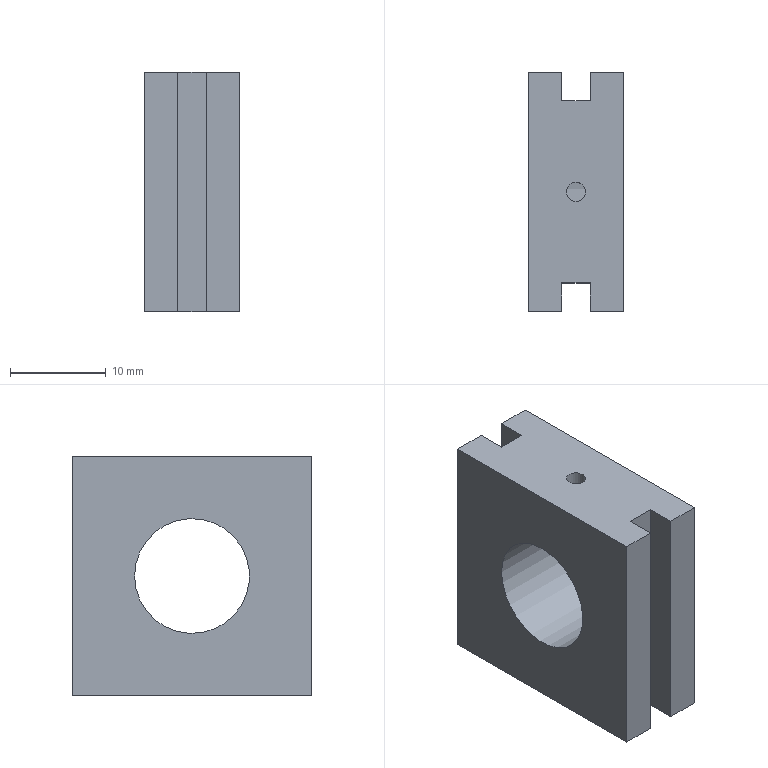Part | STEP file | 1-03.1 | 1 solid | 18 faces | box 10 x 25 x 25 mm | volume 4620 mm3 | plane 15 | cylinder 3 | commonest cylinder face diameters 2 x1 3 x1 12 x1
STEP:
#1=CARTESIAN_POINT('',(0.,0.,0.));
#2=DIRECTION('',(0.,0.,1.));
#3=DIRECTION('',(1.,0.,0.));
#4=AXIS2_PLACEMENT_3D('',#1,#2,#3);
#5=CARTESIAN_POINT('',(5.,12.5,12.5));
#6=VERTEX_POINT('',#5);
#7=CARTESIAN_POINT('',(1.5,12.5,12.5));
#8=VERTEX_POINT('',#7);
#9=CARTESIAN_POINT('',(5.,12.5,12.5));
#10=DIRECTION('',(-1.,0.,0.));
#11=VECTOR('',#10,1.);
#12=LINE('',#9,#11);
#13=CARTESIAN_POINT('',(3.25,12.5,0.));
#14=DIRECTION('',(0.,-1.,0.));
#15=DIRECTION('',(-1.,0.,0.));
#16=AXIS2_PLACEMENT_3D('',#13,#14,#15);
#17=PLANE('',#16);
#18=CARTESIAN_POINT('',(-1.75,-12.5));
#19=DIRECTION('',(1.,0.));
#20=VECTOR('',#19,1.);
#21=LINE('',#18,#20);
#22=(GEOMETRIC_REPRESENTATION_CONTEXT(2)PARAMETRIC_REPRESENTATION_CONTEXT()REPRESENTATION_CONTEXT('',''));
#23=DEFINITIONAL_REPRESENTATION('',(#21),#22);
#24=PCURVE('',#17,#23);
#25=CARTESIAN_POINT('',(-7.5,0.,12.5));
#26=DIRECTION('',(0.,0.,1.));
#27=DIRECTION('',(0.,1.,0.));
#28=AXIS2_PLACEMENT_3D('',#25,#26,#27);
#29=PLANE('',#28);
#30=CARTESIAN_POINT('',(12.5,-12.5));
#31=DIRECTION('',(0.,1.));
#32=VECTOR('',#31,1.);
#33=LINE('',#30,#32);
#34=(GEOMETRIC_REPRESENTATION_CONTEXT(2)PARAMETRIC_REPRESENTATION_CONTEXT()REPRESENTATION_CONTEXT('',''));
#35=DEFINITIONAL_REPRESENTATION('',(#33),#34);
#36=PCURVE('',#29,#35);
#37=SURFACE_CURVE('',#12,(#24,#36),.PCURVE_S1.);
#38=EDGE_CURVE('',#6,#8,#37,.T.);
#39=ORIENTED_EDGE('',*,*,#38,.T.);
#40=CARTESIAN_POINT('',(1.5,12.5,-12.5));
#41=VERTEX_POINT('',#40);
#42=CARTESIAN_POINT('',(1.5,12.5,12.5));
#43=DIRECTION('',(0.,0.,-1.));
#44=VECTOR('',#43,1.);
#45=LINE('',#42,#44);
#46=CARTESIAN_POINT('',(1.75,-12.5));
#47=DIRECTION('',(0.,1.));
#48=VECTOR('',#47,1.);
#49=LINE('',#46,#48);
#50=(GEOMETRIC_REPRESENTATION_CONTEXT(2)PARAMETRIC_REPRESENTATION_CONTEXT()REPRESENTATION_CONTEXT('',''));
#51=DEFINITIONAL_REPRESENTATION('',(#49),#50);
#52=PCURVE('',#17,#51);
#53=CARTESIAN_POINT('',(1.5,11.,0.));
#54=DIRECTION('',(1.,0.,0.));
#55=DIRECTION('',(0.,-1.,0.));
#56=AXIS2_PLACEMENT_3D('',#53,#54,#55);
#57=PLANE('',#56);
#58=CARTESIAN_POINT('',(-1.5,-12.5));
#59=DIRECTION('',(0.,1.));
#60=VECTOR('',#59,1.);
#61=LINE('',#58,#60);
#62=(GEOMETRIC_REPRESENTATION_CONTEXT(2)PARAMETRIC_REPRESENTATION_CONTEXT()REPRESENTATION_CONTEXT('',''));
#63=DEFINITIONAL_REPRESENTATION('',(#61),#62);
#64=PCURVE('',#57,#63);
#65=SURFACE_CURVE('',#45,(#52,#64),.PCURVE_S1.);
#66=EDGE_CURVE('',#8,#41,#65,.T.);
#67=ORIENTED_EDGE('',*,*,#66,.T.);
#68=CARTESIAN_POINT('',(5.,12.5,-12.5));
#69=VERTEX_POINT('',#68);
#70=CARTESIAN_POINT('',(5.,12.5,-12.5));
#71=DIRECTION('',(-1.,0.,0.));
#72=VECTOR('',#71,1.);
#73=LINE('',#70,#72);
#74=CARTESIAN_POINT('',(-1.75,12.5));
#75=DIRECTION('',(1.,0.));
#76=VECTOR('',#75,1.);
#77=LINE('',#74,#76);
#78=(GEOMETRIC_REPRESENTATION_CONTEXT(2)PARAMETRIC_REPRESENTATION_CONTEXT()REPRESENTATION_CONTEXT('',''));
#79=DEFINITIONAL_REPRESENTATION('',(#77),#78);
#80=PCURVE('',#17,#79);
#81=CARTESIAN_POINT('',(-7.5,0.,-12.5));
#82=DIRECTION('',(0.,0.,1.));
#83=DIRECTION('',(0.,1.,0.));
#84=AXIS2_PLACEMENT_3D('',#81,#82,#83);
#85=PLANE('',#84);
#86=CARTESIAN_POINT('',(12.5,-12.5));
#87=DIRECTION('',(0.,1.));
#88=VECTOR('',#87,1.);
#89=LINE('',#86,#88);
#90=(GEOMETRIC_REPRESENTATION_CONTEXT(2)PARAMETRIC_REPRESENTATION_CONTEXT()REPRESENTATION_CONTEXT('',''));
#91=DEFINITIONAL_REPRESENTATION('',(#89),#90);
#92=PCURVE('',#85,#91);
#93=SURFACE_CURVE('',#73,(#80,#92),.PCURVE_S1.);
#94=EDGE_CURVE('',#69,#41,#93,.T.);
#95=ORIENTED_EDGE('',*,*,#94,.F.);
#96=CARTESIAN_POINT('',(5.,12.5,12.5));
#97=DIRECTION('',(0.,0.,-1.));
#98=VECTOR('',#97,1.);
#99=LINE('',#96,#98);
#100=CARTESIAN_POINT('',(-1.75,-12.5));
#101=DIRECTION('',(0.,1.));
#102=VECTOR('',#101,1.);
#103=LINE('',#100,#102);
#104=(GEOMETRIC_REPRESENTATION_CONTEXT(2)PARAMETRIC_REPRESENTATION_CONTEXT()REPRESENTATION_CONTEXT('',''));
#105=DEFINITIONAL_REPRESENTATION('',(#103),#104);
#106=PCURVE('',#17,#105);
#107=CARTESIAN_POINT('',(5.,0.,0.));
#108=DIRECTION('',(-1.,0.,0.));
#109=DIRECTION('',(0.,1.,0.));
#110=AXIS2_PLACEMENT_3D('',#107,#108,#109);
#111=PLANE('',#110);
#112=CARTESIAN_POINT('',(12.5,-12.5));
#113=DIRECTION('',(0.,1.));
#114=VECTOR('',#113,1.);
#115=LINE('',#112,#114);
#116=(GEOMETRIC_REPRESENTATION_CONTEXT(2)PARAMETRIC_REPRESENTATION_CONTEXT()REPRESENTATION_CONTEXT('',''));
#117=DEFINITIONAL_REPRESENTATION('',(#115),#116);
#118=PCURVE('',#111,#117);
#119=SURFACE_CURVE('',#99,(#106,#118),.PCURVE_S1.);
#120=EDGE_CURVE('',#6,#69,#119,.T.);
#121=ORIENTED_EDGE('',*,*,#120,.F.);
#122=EDGE_LOOP('',(#39,#67,#95,#121));
#123=FACE_BOUND('',#122,.F.);
#124=ADVANCED_FACE('',(#123),#17,.F.);
#125=CARTESIAN_POINT('',(1.5,9.5,12.5));
#126=VERTEX_POINT('',#125);
#127=CARTESIAN_POINT('',(1.5,12.5,12.5));
#128=DIRECTION('',(0.,-1.,0.));
#129=VECTOR('',#128,1.);
#130=LINE('',#127,#129);
#131=CARTESIAN_POINT('',(-1.5,-12.5));
#132=DIRECTION('',(1.,0.));
#133=VECTOR('',#132,1.);
#134=LINE('',#131,#133);
#135=(GEOMETRIC_REPRESENTATION_CONTEXT(2)PARAMETRIC_REPRESENTATION_CONTEXT()REPRESENTATION_CONTEXT('',''));
#136=DEFINITIONAL_REPRESENTATION('',(#134),#135);
#137=PCURVE('',#57,#136);
#138=CARTESIAN_POINT('',(12.5,-9.));
#139=DIRECTION('',(-1.,0.));
#140=VECTOR('',#139,1.);
#141=LINE('',#138,#140);
#142=(GEOMETRIC_REPRESENTATION_CONTEXT(2)PARAMETRIC_REPRESENTATION_CONTEXT()REPRESENTATION_CONTEXT('',''));
#143=DEFINITIONAL_REPRESENTATION('',(#141),#142);
#144=PCURVE('',#29,#143);
#145=SURFACE_CURVE('',#130,(#137,#144),.PCURVE_S1.);
#146=EDGE_CURVE('',#8,#126,#145,.T.);
#147=ORIENTED_EDGE('',*,*,#146,.T.);
#148=CARTESIAN_POINT('',(1.5,9.5,-12.5));
#149=VERTEX_POINT('',#148);
#150=CARTESIAN_POINT('',(1.5,9.5,12.5));
#151=DIRECTION('',(0.,0.,-1.));
#152=VECTOR('',#151,1.);
#153=LINE('',#150,#152);
#154=CARTESIAN_POINT('',(1.5,-12.5));
#155=DIRECTION('',(0.,1.));
#156=VECTOR('',#155,1.);
#157=LINE('',#154,#156);
#158=(GEOMETRIC_REPRESENTATION_CONTEXT(2)PARAMETRIC_REPRESENTATION_CONTEXT()REPRESENTATION_CONTEXT('',''));
#159=DEFINITIONAL_REPRESENTATION('',(#157),#158);
#160=PCURVE('',#57,#159);
#161=CARTESIAN_POINT('',(0.,9.5,0.));
#162=DIRECTION('',(0.,-1.,0.));
#163=DIRECTION('',(-1.,0.,0.));
#164=AXIS2_PLACEMENT_3D('',#161,#162,#163);
#165=PLANE('',#164);
#166=CARTESIAN_POINT('',(-1.5,-12.5));
#167=DIRECTION('',(0.,1.));
#168=VECTOR('',#167,1.);
#169=LINE('',#166,#168);
#170=(GEOMETRIC_REPRESENTATION_CONTEXT(2)PARAMETRIC_REPRESENTATION_CONTEXT()REPRESENTATION_CONTEXT('',''));
#171=DEFINITIONAL_REPRESENTATION('',(#169),#170);
#172=PCURVE('',#165,#171);
#173=SURFACE_CURVE('',#153,(#160,#172),.PCURVE_S1.);
#174=EDGE_CURVE('',#126,#149,#173,.T.);
#175=ORIENTED_EDGE('',*,*,#174,.T.);
#176=CARTESIAN_POINT('',(1.5,12.5,-12.5));
#177=DIRECTION('',(0.,-1.,0.));
#178=VECTOR('',#177,1.);
#179=LINE('',#176,#178);
#180=CARTESIAN_POINT('',(-1.5,12.5));
#181=DIRECTION('',(1.,0.));
#182=VECTOR('',#181,1.);
#183=LINE('',#180,#182);
#184=(GEOMETRIC_REPRESENTATION_CONTEXT(2)PARAMETRIC_REPRESENTATION_CONTEXT()REPRESENTATION_CONTEXT('',''));
#185=DEFINITIONAL_REPRESENTATION('',(#183),#184);
#186=PCURVE('',#57,#185);
#187=CARTESIAN_POINT('',(12.5,-9.));
#188=DIRECTION('',(-1.,0.));
#189=VECTOR('',#188,1.);
#190=LINE('',#187,#189);
#191=(GEOMETRIC_REPRESENTATION_CONTEXT(2)PARAMETRIC_REPRESENTATION_CONTEXT()REPRESENTATION_CONTEXT('',''));
#192=DEFINITIONAL_REPRESENTATION('',(#190),#191);
#193=PCURVE('',#85,#192);
#194=SURFACE_CURVE('',#179,(#186,#193),.PCURVE_S1.);
#195=EDGE_CURVE('',#41,#149,#194,.T.);
#196=ORIENTED_EDGE('',*,*,#195,.F.);
#197=ORIENTED_EDGE('',*,*,#66,.F.);
#198=EDGE_LOOP('',(#147,#175,#196,#197));
#199=FACE_BOUND('',#198,.F.);
#200=ADVANCED_FACE('',(#199),#57,.F.);
#201=CARTESIAN_POINT('',(-1.5,9.5,12.5));
#202=VERTEX_POINT('',#201);
#203=CARTESIAN_POINT('',(1.5,9.5,12.5));
#204=DIRECTION('',(-1.,0.,0.));
#205=VECTOR('',#204,1.);
#206=LINE('',#203,#205);
#207=CARTESIAN_POINT('',(-1.5,-12.5));
#208=DIRECTION('',(1.,0.));
#209=VECTOR('',#208,1.);
#210=LINE('',#207,#209);
#211=(GEOMETRIC_REPRESENTATION_CONTEXT(2)PARAMETRIC_REPRESENTATION_CONTEXT()REPRESENTATION_CONTEXT('',''));
#212=DEFINITIONAL_REPRESENTATION('',(#210),#211);
#213=PCURVE('',#165,#212);
#214=CARTESIAN_POINT('',(9.5,-9.));
#215=DIRECTION('',(0.,1.));
#216=VECTOR('',#215,1.);
#217=LINE('',#214,#216);
#218=(GEOMETRIC_REPRESENTATION_CONTEXT(2)PARAMETRIC_REPRESENTATION_CONTEXT()REPRESENTATION_CONTEXT('',''));
#219=DEFINITIONAL_REPRESENTATION('',(#217),#218);
#220=PCURVE('',#29,#219);
#221=SURFACE_CURVE('',#206,(#213,#220),.PCURVE_S1.);
#222=EDGE_CURVE('',#126,#202,#221,.T.);
#223=ORIENTED_EDGE('',*,*,#222,.T.);
#224=CARTESIAN_POINT('',(-1.5,9.5,-12.5));
#225=VERTEX_POINT('',#224);
#226=CARTESIAN_POINT('',(-1.5,9.5,12.5));
#227=DIRECTION('',(0.,0.,-1.));
#228=VECTOR('',#227,1.);
#229=LINE('',#226,#228);
#230=CARTESIAN_POINT('',(1.5,-12.5));
#231=DIRECTION('',(0.,1.));
#232=VECTOR('',#231,1.);
#233=LINE('',#230,#232);
#234=(GEOMETRIC_REPRESENTATION_CONTEXT(2)PARAMETRIC_REPRESENTATION_CONTEXT()REPRESENTATION_CONTEXT('',''));
#235=DEFINITIONAL_REPRESENTATION('',(#233),#234);
#236=PCURVE('',#165,#235);
#237=CARTESIAN_POINT('',(-1.5,11.,0.));
#238=DIRECTION('',(-1.,0.,0.));
#239=DIRECTION('',(0.,1.,0.));
#240=AXIS2_PLACEMENT_3D('',#237,#238,#239);
#241=PLANE('',#240);
#242=CARTESIAN_POINT('',(-1.5,-12.5));
#243=DIRECTION('',(0.,1.));
#244=VECTOR('',#243,1.);
#245=LINE('',#242,#244);
#246=(GEOMETRIC_REPRESENTATION_CONTEXT(2)PARAMETRIC_REPRESENTATION_CONTEXT()REPRESENTATION_CONTEXT('',''));
#247=DEFINITIONAL_REPRESENTATION('',(#245),#246);
#248=PCURVE('',#241,#247);
#249=SURFACE_CURVE('',#229,(#236,#248),.PCURVE_S1.);
#250=EDGE_CURVE('',#202,#225,#249,.T.);
#251=ORIENTED_EDGE('',*,*,#250,.T.);
#252=CARTESIAN_POINT('',(1.5,9.5,-12.5));
#253=DIRECTION('',(-1.,0.,0.));
#254=VECTOR('',#253,1.);
#255=LINE('',#252,#254);
#256=CARTESIAN_POINT('',(-1.5,12.5));
#257=DIRECTION('',(1.,0.));
#258=VECTOR('',#257,1.);
#259=LINE('',#256,#258);
#260=(GEOMETRIC_REPRESENTATION_CONTEXT(2)PARAMETRIC_REPRESENTATION_CONTEXT()REPRESENTATION_CONTEXT('',''));
#261=DEFINITIONAL_REPRESENTATION('',(#259),#260);
#262=PCURVE('',#165,#261);
#263=CARTESIAN_POINT('',(9.5,-9.));
#264=DIRECTION('',(0.,1.));
#265=VECTOR('',#264,1.);
#266=LINE('',#263,#265);
#267=(GEOMETRIC_REPRESENTATION_CONTEXT(2)PARAMETRIC_REPRESENTATION_CONTEXT()REPRESENTATION_CONTEXT('',''));
#268=DEFINITIONAL_REPRESENTATION('',(#266),#267);
#269=PCURVE('',#85,#268);
#270=SURFACE_CURVE('',#255,(#262,#269),.PCURVE_S1.);
#271=EDGE_CURVE('',#149,#225,#270,.T.);
#272=ORIENTED_EDGE('',*,*,#271,.F.);
#273=ORIENTED_EDGE('',*,*,#174,.F.);
#274=EDGE_LOOP('',(#223,#251,#272,#273));
#275=FACE_BOUND('',#274,.F.);
#276=ADVANCED_FACE('',(#275),#165,.F.);
#277=CARTESIAN_POINT('',(-1.5,12.5,12.5));
#278=VERTEX_POINT('',#277);
#279=CARTESIAN_POINT('',(-1.5,9.5,12.5));
#280=DIRECTION('',(0.,1.,0.));
#281=VECTOR('',#280,1.);
#282=LINE('',#279,#281);
#283=CARTESIAN_POINT('',(-1.5,-12.5));
#284=DIRECTION('',(1.,0.));
#285=VECTOR('',#284,1.);
#286=LINE('',#283,#285);
#287=(GEOMETRIC_REPRESENTATION_CONTEXT(2)PARAMETRIC_REPRESENTATION_CONTEXT()REPRESENTATION_CONTEXT('',''));
#288=DEFINITIONAL_REPRESENTATION('',(#286),#287);
#289=PCURVE('',#241,#288);
#290=CARTESIAN_POINT('',(9.5,-6.));
#291=DIRECTION('',(1.,0.));
#292=VECTOR('',#291,1.);
#293=LINE('',#290,#292);
#294=(GEOMETRIC_REPRESENTATION_CONTEXT(2)PARAMETRIC_REPRESENTATION_CONTEXT()REPRESENTATION_CONTEXT('',''));
#295=DEFINITIONAL_REPRESENTATION('',(#293),#294);
#296=PCURVE('',#29,#295);
#297=SURFACE_CURVE('',#282,(#289,#296),.PCURVE_S1.);
#298=EDGE_CURVE('',#202,#278,#297,.T.);
#299=ORIENTED_EDGE('',*,*,#298,.T.);
#300=CARTESIAN_POINT('',(-1.5,12.5,-12.5));
#301=VERTEX_POINT('',#300);
#302=CARTESIAN_POINT('',(-1.5,12.5,12.5));
#303=DIRECTION('',(0.,0.,-1.));
#304=VECTOR('',#303,1.);
#305=LINE('',#302,#304);
#306=CARTESIAN_POINT('',(1.5,-12.5));
#307=DIRECTION('',(0.,1.));
#308=VECTOR('',#307,1.);
#309=LINE('',#306,#308);
#310=(GEOMETRIC_REPRESENTATION_CONTEXT(2)PARAMETRIC_REPRESENTATION_CONTEXT()REPRESENTATION_CONTEXT('',''));
#311=DEFINITIONAL_REPRESENTATION('',(#309),#310);
#312=PCURVE('',#241,#311);
#313=CARTESIAN_POINT('',(-3.25,12.5,0.));
#314=DIRECTION('',(0.,-1.,0.));
#315=DIRECTION('',(-1.,0.,0.));
#316=AXIS2_PLACEMENT_3D('',#313,#314,#315);
#317=PLANE('',#316);
#318=CARTESIAN_POINT('',(-1.75,-12.5));
#319=DIRECTION('',(0.,1.));
#320=VECTOR('',#319,1.);
#321=LINE('',#318,#320);
#322=(GEOMETRIC_REPRESENTATION_CONTEXT(2)PARAMETRIC_REPRESENTATION_CONTEXT()REPRESENTATION_CONTEXT('',''));
#323=DEFINITIONAL_REPRESENTATION('',(#321),#322);
#324=PCURVE('',#317,#323);
#325=SURFACE_CURVE('',#305,(#312,#324),.PCURVE_S1.);
#326=EDGE_CURVE('',#278,#301,#325,.T.);
#327=ORIENTED_EDGE('',*,*,#326,.T.);
#328=CARTESIAN_POINT('',(-1.5,9.5,-12.5));
#329=DIRECTION('',(0.,1.,0.));
#330=VECTOR('',#329,1.);
#331=LINE('',#328,#330);
#332=CARTESIAN_POINT('',(-1.5,12.5));
#333=DIRECTION('',(1.,0.));
#334=VECTOR('',#333,1.);
#335=LINE('',#332,#334);
#336=(GEOMETRIC_REPRESENTATION_CONTEXT(2)PARAMETRIC_REPRESENTATION_CONTEXT()REPRESENTATION_CONTEXT('',''));
#337=DEFINITIONAL_REPRESENTATION('',(#335),#336);
#338=PCURVE('',#241,#337);
#339=CARTESIAN_POINT('',(9.5,-6.));
#340=DIRECTION('',(1.,0.));
#341=VECTOR('',#340,1.);
#342=LINE('',#339,#341);
#343=(GEOMETRIC_REPRESENTATION_CONTEXT(2)PARAMETRIC_REPRESENTATION_CONTEXT()REPRESENTATION_CONTEXT('',''));
#344=DEFINITIONAL_REPRESENTATION('',(#342),#343);
#345=PCURVE('',#85,#344);
#346=SURFACE_CURVE('',#331,(#338,#345),.PCURVE_S1.);
#347=EDGE_CURVE('',#225,#301,#346,.T.);
#348=ORIENTED_EDGE('',*,*,#347,.F.);
#349=ORIENTED_EDGE('',*,*,#250,.F.);
#350=EDGE_LOOP('',(#299,#327,#348,#349));
#351=FACE_BOUND('',#350,.F.);
#352=ADVANCED_FACE('',(#351),#241,.F.);
#353=CARTESIAN_POINT('',(-5.,12.5,12.5));
#354=VERTEX_POINT('',#353);
#355=CARTESIAN_POINT('',(-1.5,12.5,12.5));
#356=DIRECTION('',(-1.,0.,0.));
#357=VECTOR('',#356,1.);
#358=LINE('',#355,#357);
#359=CARTESIAN_POINT('',(-1.75,-12.5));
#360=DIRECTION('',(1.,0.));
#361=VECTOR('',#360,1.);
#362=LINE('',#359,#361);
#363=(GEOMETRIC_REPRESENTATION_CONTEXT(2)PARAMETRIC_REPRESENTATION_CONTEXT()REPRESENTATION_CONTEXT('',''));
#364=DEFINITIONAL_REPRESENTATION('',(#362),#363);
#365=PCURVE('',#317,#364);
#366=CARTESIAN_POINT('',(12.5,-6.));
#367=DIRECTION('',(0.,1.));
#368=VECTOR('',#367,1.);
#369=LINE('',#366,#368);
#370=(GEOMETRIC_REPRESENTATION_CONTEXT(2)PARAMETRIC_REPRESENTATION_CONTEXT()REPRESENTATION_CONTEXT('',''));
#371=DEFINITIONAL_REPRESENTATION('',(#369),#370);
#372=PCURVE('',#29,#371);
#373=SURFACE_CURVE('',#358,(#365,#372),.PCURVE_S1.);
#374=EDGE_CURVE('',#278,#354,#373,.T.);
#375=ORIENTED_EDGE('',*,*,#374,.T.);
#376=CARTESIAN_POINT('',(-5.,12.5,-12.5));
#377=VERTEX_POINT('',#376);
#378=CARTESIAN_POINT('',(-5.,12.5,12.5));
#379=DIRECTION('',(0.,0.,-1.));
#380=VECTOR('',#379,1.);
#381=LINE('',#378,#380);
#382=CARTESIAN_POINT('',(1.75,-12.5));
#383=DIRECTION('',(0.,1.));
#384=VECTOR('',#383,1.);
#385=LINE('',#382,#384);
#386=(GEOMETRIC_REPRESENTATION_CONTEXT(2)PARAMETRIC_REPRESENTATION_CONTEXT()REPRESENTATION_CONTEXT('',''));
#387=DEFINITIONAL_REPRESENTATION('',(#385),#386);
#388=PCURVE('',#317,#387);
#389=CARTESIAN_POINT('',(-5.,0.,0.));
#390=DIRECTION('',(1.,0.,0.));
#391=DIRECTION('',(0.,-1.,0.));
#392=AXIS2_PLACEMENT_3D('',#389,#390,#391);
#393=PLANE('',#392);
#394=CARTESIAN_POINT('',(-12.5,-12.5));
#395=DIRECTION('',(0.,1.));
#396=VECTOR('',#395,1.);
#397=LINE('',#394,#396);
#398=(GEOMETRIC_REPRESENTATION_CONTEXT(2)PARAMETRIC_REPRESENTATION_CONTEXT()REPRESENTATION_CONTEXT('',''));
#399=DEFINITIONAL_REPRESENTATION('',(#397),#398);
#400=PCURVE('',#393,#399);
#401=SURFACE_CURVE('',#381,(#388,#400),.PCURVE_S1.);
#402=EDGE_CURVE('',#354,#377,#401,.T.);
#403=ORIENTED_EDGE('',*,*,#402,.T.);
#404=CARTESIAN_POINT('',(-1.5,12.5,-12.5));
#405=DIRECTION('',(-1.,0.,0.));
#406=VECTOR('',#405,1.);
#407=LINE('',#404,#406);
#408=CARTESIAN_POINT('',(-1.75,12.5));
#409=DIRECTION('',(1.,0.));
#410=VECTOR('',#409,1.);
#411=LINE('',#408,#410);
#412=(GEOMETRIC_REPRESENTATION_CONTEXT(2)PARAMETRIC_REPRESENTATION_CONTEXT()REPRESENTATION_CONTEXT('',''));
#413=DEFINITIONAL_REPRESENTATION('',(#411),#412);
#414=PCURVE('',#317,#413);
#415=CARTESIAN_POINT('',(12.5,-6.));
#416=DIRECTION('',(0.,1.));
#417=VECTOR('',#416,1.);
#418=LINE('',#415,#417);
#419=(GEOMETRIC_REPRESENTATION_CONTEXT(2)PARAMETRIC_REPRESENTATION_CONTEXT()REPRESENTATION_CONTEXT('',''));
#420=DEFINITIONAL_REPRESENTATION('',(#418),#419);
#421=PCURVE('',#85,#420);
#422=SURFACE_CURVE('',#407,(#414,#421),.PCURVE_S1.);
#423=EDGE_CURVE('',#301,#377,#422,.T.);
#424=ORIENTED_EDGE('',*,*,#423,.F.);
#425=ORIENTED_EDGE('',*,*,#326,.F.);
#426=EDGE_LOOP('',(#375,#403,#424,#425));
#427=FACE_BOUND('',#426,.F.);
#428=ADVANCED_FACE('',(#427),#317,.F.);
#429=CARTESIAN_POINT('',(-5.,-12.5,12.5));
#430=VERTEX_POINT('',#429);
#431=CARTESIAN_POINT('',(-1.5,-12.5,12.5));
#432=VERTEX_POINT('',#431);
#433=CARTESIAN_POINT('',(-5.,-12.5,12.5));
#434=DIRECTION('',(1.,0.,0.));
#435=VECTOR('',#434,1.);
#436=LINE('',#433,#435);
#437=CARTESIAN_POINT('',(-3.25,-12.5,0.));
#438=DIRECTION('',(0.,1.,0.));
#439=DIRECTION('',(1.,0.,0.));
#440=AXIS2_PLACEMENT_3D('',#437,#438,#439);
#441=PLANE('',#440);
#442=CARTESIAN_POINT('',(-1.75,-12.5));
#443=DIRECTION('',(1.,0.));
#444=VECTOR('',#443,1.);
#445=LINE('',#442,#444);
#446=(GEOMETRIC_REPRESENTATION_CONTEXT(2)PARAMETRIC_REPRESENTATION_CONTEXT()REPRESENTATION_CONTEXT('',''));
#447=DEFINITIONAL_REPRESENTATION('',(#445),#446);
#448=PCURVE('',#441,#447);
#449=CARTESIAN_POINT('',(-12.5,-2.5));
#450=DIRECTION('',(0.,-1.));
#451=VECTOR('',#450,1.);
#452=LINE('',#449,#451);
#453=(GEOMETRIC_REPRESENTATION_CONTEXT(2)PARAMETRIC_REPRESENTATION_CONTEXT()REPRESENTATION_CONTEXT('',''));
#454=DEFINITIONAL_REPRESENTATION('',(#452),#453);
#455=PCURVE('',#29,#454);
#456=SURFACE_CURVE('',#436,(#448,#455),.PCURVE_S1.);
#457=EDGE_CURVE('',#430,#432,#456,.T.);
#458=ORIENTED_EDGE('',*,*,#457,.T.);
#459=CARTESIAN_POINT('',(-1.5,-12.5,-12.5));
#460=VERTEX_POINT('',#459);
#461=CARTESIAN_POINT('',(-1.5,-12.5,12.5));
#462=DIRECTION('',(0.,0.,-1.));
#463=VECTOR('',#462,1.);
#464=LINE('',#461,#463);
#465=CARTESIAN_POINT('',(1.75,-12.5));
#466=DIRECTION('',(0.,1.));
#467=VECTOR('',#466,1.);
#468=LINE('',#465,#467);
#469=(GEOMETRIC_REPRESENTATION_CONTEXT(2)PARAMETRIC_REPRESENTATION_CONTEXT()REPRESENTATION_CONTEXT('',''));
#470=DEFINITIONAL_REPRESENTATION('',(#468),#469);
#471=PCURVE('',#441,#470);
#472=CARTESIAN_POINT('',(-1.5,-11.,0.));
#473=DIRECTION('',(-1.,0.,0.));
#474=DIRECTION('',(0.,1.,0.));
#475=AXIS2_PLACEMENT_3D('',#472,#473,#474);
#476=PLANE('',#475);
#477=CARTESIAN_POINT('',(-1.5,-12.5));
#478=DIRECTION('',(0.,1.));
#479=VECTOR('',#478,1.);
#480=LINE('',#477,#479);
#481=(GEOMETRIC_REPRESENTATION_CONTEXT(2)PARAMETRIC_REPRESENTATION_CONTEXT()REPRESENTATION_CONTEXT('',''));
#482=DEFINITIONAL_REPRESENTATION('',(#480),#481);
#483=PCURVE('',#476,#482);
#484=SURFACE_CURVE('',#464,(#471,#483),.PCURVE_S1.);
#485=EDGE_CURVE('',#432,#460,#484,.T.);
#486=ORIENTED_EDGE('',*,*,#485,.T.);
#487=CARTESIAN_POINT('',(-5.,-12.5,-12.5));
#488=VERTEX_POINT('',#487);
#489=CARTESIAN_POINT('',(-5.,-12.5,-12.5));
#490=DIRECTION('',(1.,0.,0.));
#491=VECTOR('',#490,1.);
#492=LINE('',#489,#491);
#493=CARTESIAN_POINT('',(-1.75,12.5));
#494=DIRECTION('',(1.,0.));
#495=VECTOR('',#494,1.);
#496=LINE('',#493,#495);
#497=(GEOMETRIC_REPRESENTATION_CONTEXT(2)PARAMETRIC_REPRESENTATION_CONTEXT()REPRESENTATION_CONTEXT('',''));
#498=DEFINITIONAL_REPRESENTATION('',(#496),#497);
#499=PCURVE('',#441,#498);
#500=CARTESIAN_POINT('',(-12.5,-2.5));
#501=DIRECTION('',(0.,-1.));
#502=VECTOR('',#501,1.);
#503=LINE('',#500,#502);
#504=(GEOMETRIC_REPRESENTATION_CONTEXT(2)PARAMETRIC_REPRESENTATION_CONTEXT()REPRESENTATION_CONTEXT('',''));
#505=DEFINITIONAL_REPRESENTATION('',(#503),#504);
#506=PCURVE('',#85,#505);
#507=SURFACE_CURVE('',#492,(#499,#506),.PCURVE_S1.);
#508=EDGE_CURVE('',#488,#460,#507,.T.);
#509=ORIENTED_EDGE('',*,*,#508,.F.);
#510=CARTESIAN_POINT('',(-5.,-12.5,12.5));
#511=DIRECTION('',(0.,0.,-1.));
#512=VECTOR('',#511,1.);
#513=LINE('',#510,#512);
#514=CARTESIAN_POINT('',(-1.75,-12.5));
#515=DIRECTION('',(0.,1.));
#516=VECTOR('',#515,1.);
#517=LINE('',#514,#516);
#518=(GEOMETRIC_REPRESENTATION_CONTEXT(2)PARAMETRIC_REPRESENTATION_CONTEXT()REPRESENTATION_CONTEXT('',''));
#519=DEFINITIONAL_REPRESENTATION('',(#517),#518);
#520=PCURVE('',#441,#519);
#521=CARTESIAN_POINT('',(12.5,-12.5));
#522=DIRECTION('',(0.,1.));
#523=VECTOR('',#522,1.);
#524=LINE('',#521,#523);
#525=(GEOMETRIC_REPRESENTATION_CONTEXT(2)PARAMETRIC_REPRESENTATION_CONTEXT()REPRESENTATION_CONTEXT('',''));
#526=DEFINITIONAL_REPRESENTATION('',(#524),#525);
#527=PCURVE('',#393,#526);
#528=SURFACE_CURVE('',#513,(#520,#527),.PCURVE_S1.);
#529=EDGE_CURVE('',#430,#488,#528,.T.);
#530=ORIENTED_EDGE('',*,*,#529,.F.);
#531=EDGE_LOOP('',(#458,#486,#509,#530));
#532=FACE_BOUND('',#531,.F.);
#533=ADVANCED_FACE('',(#532),#441,.F.);
#534=CARTESIAN_POINT('',(-1.5,-9.5,12.5));
#535=VERTEX_POINT('',#534);
#536=CARTESIAN_POINT('',(-1.5,-12.5,12.5));
#537=DIRECTION('',(0.,1.,0.));
#538=VECTOR('',#537,1.);
#539=LINE('',#536,#538);
#540=CARTESIAN_POINT('',(-1.5,-12.5));
#541=DIRECTION('',(1.,0.));
#542=VECTOR('',#541,1.);
#543=LINE('',#540,#542);
#544=(GEOMETRIC_REPRESENTATION_CONTEXT(2)PARAMETRIC_REPRESENTATION_CONTEXT()REPRESENTATION_CONTEXT('',''));
#545=DEFINITIONAL_REPRESENTATION('',(#543),#544);
#546=PCURVE('',#476,#545);
#547=CARTESIAN_POINT('',(-12.5,-6.));
#548=DIRECTION('',(1.,0.));
#549=VECTOR('',#548,1.);
#550=LINE('',#547,#549);
#551=(GEOMETRIC_REPRESENTATION_CONTEXT(2)PARAMETRIC_REPRESENTATION_CONTEXT()REPRESENTATION_CONTEXT('',''));
#552=DEFINITIONAL_REPRESENTATION('',(#550),#551);
#553=PCURVE('',#29,#552);
#554=SURFACE_CURVE('',#539,(#546,#553),.PCURVE_S1.);
#555=EDGE_CURVE('',#432,#535,#554,.T.);
#556=ORIENTED_EDGE('',*,*,#555,.T.);
#557=CARTESIAN_POINT('',(-1.5,-9.5,-12.5));
#558=VERTEX_POINT('',#557);
#559=CARTESIAN_POINT('',(-1.5,-9.5,12.5));
#560=DIRECTION('',(0.,0.,-1.));
#561=VECTOR('',#560,1.);
#562=LINE('',#559,#561);
#563=CARTESIAN_POINT('',(1.5,-12.5));
#564=DIRECTION('',(0.,1.));
#565=VECTOR('',#564,1.);
#566=LINE('',#563,#565);
#567=(GEOMETRIC_REPRESENTATION_CONTEXT(2)PARAMETRIC_REPRESENTATION_CONTEXT()REPRESENTATION_CONTEXT('',''));
#568=DEFINITIONAL_REPRESENTATION('',(#566),#567);
#569=PCURVE('',#476,#568);
#570=CARTESIAN_POINT('',(0.,-9.5,0.));
#571=DIRECTION('',(0.,1.,0.));
#572=DIRECTION('',(1.,0.,0.));
#573=AXIS2_PLACEMENT_3D('',#570,#571,#572);
#574=PLANE('',#573);
#575=CARTESIAN_POINT('',(-1.5,-12.5));
#576=DIRECTION('',(0.,1.));
#577=VECTOR('',#576,1.);
#578=LINE('',#575,#577);
#579=(GEOMETRIC_REPRESENTATION_CONTEXT(2)PARAMETRIC_REPRESENTATION_CONTEXT()REPRESENTATION_CONTEXT('',''));
#580=DEFINITIONAL_REPRESENTATION('',(#578),#579);
#581=PCURVE('',#574,#580);
#582=SURFACE_CURVE('',#562,(#569,#581),.PCURVE_S1.);
#583=EDGE_CURVE('',#535,#558,#582,.T.);
#584=ORIENTED_EDGE('',*,*,#583,.T.);
#585=CARTESIAN_POINT('',(-1.5,-12.5,-12.5));
#586=DIRECTION('',(0.,1.,0.));
#587=VECTOR('',#586,1.);
#588=LINE('',#585,#587);
#589=CARTESIAN_POINT('',(-1.5,12.5));
#590=DIRECTION('',(1.,0.));
#591=VECTOR('',#590,1.);
#592=LINE('',#589,#591);
#593=(GEOMETRIC_REPRESENTATION_CONTEXT(2)PARAMETRIC_REPRESENTATION_CONTEXT()REPRESENTATION_CONTEXT('',''));
#594=DEFINITIONAL_REPRESENTATION('',(#592),#593);
#595=PCURVE('',#476,#594);
#596=CARTESIAN_POINT('',(-12.5,-6.));
#597=DIRECTION('',(1.,0.));
#598=VECTOR('',#597,1.);
#599=LINE('',#596,#598);
#600=(GEOMETRIC_REPRESENTATION_CONTEXT(2)PARAMETRIC_REPRESENTATION_CONTEXT()REPRESENTATION_CONTEXT('',''));
#601=DEFINITIONAL_REPRESENTATION('',(#599),#600);
#602=PCURVE('',#85,#601);
#603=SURFACE_CURVE('',#588,(#595,#602),.PCURVE_S1.);
#604=EDGE_CURVE('',#460,#558,#603,.T.);
#605=ORIENTED_EDGE('',*,*,#604,.F.);
#606=ORIENTED_EDGE('',*,*,#485,.F.);
#607=EDGE_LOOP('',(#556,#584,#605,#606));
#608=FACE_BOUND('',#607,.F.);
#609=ADVANCED_FACE('',(#608),#476,.F.);
#610=CARTESIAN_POINT('',(1.5,-9.5,12.5));
#611=VERTEX_POINT('',#610);
#612=CARTESIAN_POINT('',(-1.5,-9.5,12.5));
#613=DIRECTION('',(1.,0.,0.));
#614=VECTOR('',#613,1.);
#615=LINE('',#612,#614);
#616=CARTESIAN_POINT('',(-1.5,-12.5));
#617=DIRECTION('',(1.,0.));
#618=VECTOR('',#617,1.);
#619=LINE('',#616,#618);
#620=(GEOMETRIC_REPRESENTATION_CONTEXT(2)PARAMETRIC_REPRESENTATION_CONTEXT()REPRESENTATION_CONTEXT('',''));
#621=DEFINITIONAL_REPRESENTATION('',(#619),#620);
#622=PCURVE('',#574,#621);
#623=CARTESIAN_POINT('',(-9.5,-6.));
#624=DIRECTION('',(0.,-1.));
#625=VECTOR('',#624,1.);
#626=LINE('',#623,#625);
#627=(GEOMETRIC_REPRESENTATION_CONTEXT(2)PARAMETRIC_REPRESENTATION_CONTEXT()REPRESENTATION_CONTEXT('',''));
#628=DEFINITIONAL_REPRESENTATION('',(#626),#627);
#629=PCURVE('',#29,#628);
#630=SURFACE_CURVE('',#615,(#622,#629),.PCURVE_S1.);
#631=EDGE_CURVE('',#535,#611,#630,.T.);
#632=ORIENTED_EDGE('',*,*,#631,.T.);
#633=CARTESIAN_POINT('',(1.5,-9.5,-12.5));
#634=VERTEX_POINT('',#633);
#635=CARTESIAN_POINT('',(1.5,-9.5,12.5));
#636=DIRECTION('',(0.,0.,-1.));
#637=VECTOR('',#636,1.);
#638=LINE('',#635,#637);
#639=CARTESIAN_POINT('',(1.5,-12.5));
#640=DIRECTION('',(0.,1.));
#641=VECTOR('',#640,1.);
#642=LINE('',#639,#641);
#643=(GEOMETRIC_REPRESENTATION_CONTEXT(2)PARAMETRIC_REPRESENTATION_CONTEXT()REPRESENTATION_CONTEXT('',''));
#644=DEFINITIONAL_REPRESENTATION('',(#642),#643);
#645=PCURVE('',#574,#644);
#646=CARTESIAN_POINT('',(1.5,-11.,0.));
#647=DIRECTION('',(1.,0.,0.));
#648=DIRECTION('',(0.,-1.,0.));
#649=AXIS2_PLACEMENT_3D('',#646,#647,#648);
#650=PLANE('',#649);
#651=CARTESIAN_POINT('',(-1.5,-12.5));
#652=DIRECTION('',(0.,1.));
#653=VECTOR('',#652,1.);
#654=LINE('',#651,#653);
#655=(GEOMETRIC_REPRESENTATION_CONTEXT(2)PARAMETRIC_REPRESENTATION_CONTEXT()REPRESENTATION_CONTEXT('',''));
#656=DEFINITIONAL_REPRESENTATION('',(#654),#655);
#657=PCURVE('',#650,#656);
#658=SURFACE_CURVE('',#638,(#645,#657),.PCURVE_S1.);
#659=EDGE_CURVE('',#611,#634,#658,.T.);
#660=ORIENTED_EDGE('',*,*,#659,.T.);
#661=CARTESIAN_POINT('',(-1.5,-9.5,-12.5));
#662=DIRECTION('',(1.,0.,0.));
#663=VECTOR('',#662,1.);
#664=LINE('',#661,#663);
#665=CARTESIAN_POINT('',(-1.5,12.5));
#666=DIRECTION('',(1.,0.));
#667=VECTOR('',#666,1.);
#668=LINE('',#665,#667);
#669=(GEOMETRIC_REPRESENTATION_CONTEXT(2)PARAMETRIC_REPRESENTATION_CONTEXT()REPRESENTATION_CONTEXT('',''));
#670=DEFINITIONAL_REPRESENTATION('',(#668),#669);
#671=PCURVE('',#574,#670);
#672=CARTESIAN_POINT('',(-9.5,-6.));
#673=DIRECTION('',(0.,-1.));
#674=VECTOR('',#673,1.);
#675=LINE('',#672,#674);
#676=(GEOMETRIC_REPRESENTATION_CONTEXT(2)PARAMETRIC_REPRESENTATION_CONTEXT()REPRESENTATION_CONTEXT('',''));
#677=DEFINITIONAL_REPRESENTATION('',(#675),#676);
#678=PCURVE('',#85,#677);
#679=SURFACE_CURVE('',#664,(#671,#678),.PCURVE_S1.);
#680=EDGE_CURVE('',#558,#634,#679,.T.);
#681=ORIENTED_EDGE('',*,*,#680,.F.);
#682=ORIENTED_EDGE('',*,*,#583,.F.);
#683=EDGE_LOOP('',(#632,#660,#681,#682));
#684=FACE_BOUND('',#683,.F.);
#685=ADVANCED_FACE('',(#684),#574,.F.);
#686=CARTESIAN_POINT('',(1.5,-12.5,12.5));
#687=VERTEX_POINT('',#686);
#688=CARTESIAN_POINT('',(1.5,-9.5,12.5));
#689=DIRECTION('',(0.,-1.,0.));
#690=VECTOR('',#689,1.);
#691=LINE('',#688,#690);
#692=CARTESIAN_POINT('',(-1.5,-12.5));
#693=DIRECTION('',(1.,0.));
#694=VECTOR('',#693,1.);
#695=LINE('',#692,#694);
#696=(GEOMETRIC_REPRESENTATION_CONTEXT(2)PARAMETRIC_REPRESENTATION_CONTEXT()REPRESENTATION_CONTEXT('',''));
#697=DEFINITIONAL_REPRESENTATION('',(#695),#696);
#698=PCURVE('',#650,#697);
#699=CARTESIAN_POINT('',(-9.5,-9.));
#700=DIRECTION('',(-1.,0.));
#701=VECTOR('',#700,1.);
#702=LINE('',#699,#701);
#703=(GEOMETRIC_REPRESENTATION_CONTEXT(2)PARAMETRIC_REPRESENTATION_CONTEXT()REPRESENTATION_CONTEXT('',''));
#704=DEFINITIONAL_REPRESENTATION('',(#702),#703);
#705=PCURVE('',#29,#704);
#706=SURFACE_CURVE('',#691,(#698,#705),.PCURVE_S1.);
#707=EDGE_CURVE('',#611,#687,#706,.T.);
#708=ORIENTED_EDGE('',*,*,#707,.T.);
#709=CARTESIAN_POINT('',(1.5,-12.5,-12.5));
#710=VERTEX_POINT('',#709);
#711=CARTESIAN_POINT('',(1.5,-12.5,12.5));
#712=DIRECTION('',(0.,0.,-1.));
#713=VECTOR('',#712,1.);
#714=LINE('',#711,#713);
#715=CARTESIAN_POINT('',(1.5,-12.5));
#716=DIRECTION('',(0.,1.));
#717=VECTOR('',#716,1.);
#718=LINE('',#715,#717);
#719=(GEOMETRIC_REPRESENTATION_CONTEXT(2)PARAMETRIC_REPRESENTATION_CONTEXT()REPRESENTATION_CONTEXT('',''));
#720=DEFINITIONAL_REPRESENTATION('',(#718),#719);
#721=PCURVE('',#650,#720);
#722=CARTESIAN_POINT('',(3.25,-12.5,0.));
#723=DIRECTION('',(0.,1.,0.));
#724=DIRECTION('',(1.,0.,0.));
#725=AXIS2_PLACEMENT_3D('',#722,#723,#724);
#726=PLANE('',#725);
#727=CARTESIAN_POINT('',(-1.75,-12.5));
#728=DIRECTION('',(0.,1.));
#729=VECTOR('',#728,1.);
#730=LINE('',#727,#729);
#731=(GEOMETRIC_REPRESENTATION_CONTEXT(2)PARAMETRIC_REPRESENTATION_CONTEXT()REPRESENTATION_CONTEXT('',''));
#732=DEFINITIONAL_REPRESENTATION('',(#730),#731);
#733=PCURVE('',#726,#732);
#734=SURFACE_CURVE('',#714,(#721,#733),.PCURVE_S1.);
#735=EDGE_CURVE('',#687,#710,#734,.T.);
#736=ORIENTED_EDGE('',*,*,#735,.T.);
#737=CARTESIAN_POINT('',(1.5,-9.5,-12.5));
#738=DIRECTION('',(0.,-1.,0.));
#739=VECTOR('',#738,1.);
#740=LINE('',#737,#739);
#741=CARTESIAN_POINT('',(-1.5,12.5));
#742=DIRECTION('',(1.,0.));
#743=VECTOR('',#742,1.);
#744=LINE('',#741,#743);
#745=(GEOMETRIC_REPRESENTATION_CONTEXT(2)PARAMETRIC_REPRESENTATION_CONTEXT()REPRESENTATION_CONTEXT('',''));
#746=DEFINITIONAL_REPRESENTATION('',(#744),#745);
#747=PCURVE('',#650,#746);
#748=CARTESIAN_POINT('',(-9.5,-9.));
#749=DIRECTION('',(-1.,0.));
#750=VECTOR('',#749,1.);
#751=LINE('',#748,#750);
#752=(GEOMETRIC_REPRESENTATION_CONTEXT(2)PARAMETRIC_REPRESENTATION_CONTEXT()REPRESENTATION_CONTEXT('',''));
#753=DEFINITIONAL_REPRESENTATION('',(#751),#752);
#754=PCURVE('',#85,#753);
#755=SURFACE_CURVE('',#740,(#747,#754),.PCURVE_S1.);
#756=EDGE_CURVE('',#634,#710,#755,.T.);
#757=ORIENTED_EDGE('',*,*,#756,.F.);
#758=ORIENTED_EDGE('',*,*,#659,.F.);
#759=EDGE_LOOP('',(#708,#736,#757,#758));
#760=FACE_BOUND('',#759,.F.);
#761=ADVANCED_FACE('',(#760),#650,.F.);
#762=CARTESIAN_POINT('',(5.,-12.5,12.5));
#763=VERTEX_POINT('',#762);
#764=CARTESIAN_POINT('',(1.5,-12.5,12.5));
#765=DIRECTION('',(1.,0.,0.));
#766=VECTOR('',#765,1.);
#767=LINE('',#764,#766);
#768=CARTESIAN_POINT('',(-1.75,-12.5));
#769=DIRECTION('',(1.,0.));
#770=VECTOR('',#769,1.);
#771=LINE('',#768,#770);
#772=(GEOMETRIC_REPRESENTATION_CONTEXT(2)PARAMETRIC_REPRESENTATION_CONTEXT()REPRESENTATION_CONTEXT('',''));
#773=DEFINITIONAL_REPRESENTATION('',(#771),#772);
#774=PCURVE('',#726,#773);
#775=CARTESIAN_POINT('',(-12.5,-9.));
#776=DIRECTION('',(0.,-1.));
#777=VECTOR('',#776,1.);
#778=LINE('',#775,#777);
#779=(GEOMETRIC_REPRESENTATION_CONTEXT(2)PARAMETRIC_REPRESENTATION_CONTEXT()REPRESENTATION_CONTEXT('',''));
#780=DEFINITIONAL_REPRESENTATION('',(#778),#779);
#781=PCURVE('',#29,#780);
#782=SURFACE_CURVE('',#767,(#774,#781),.PCURVE_S1.);
#783=EDGE_CURVE('',#687,#763,#782,.T.);
#784=ORIENTED_EDGE('',*,*,#783,.T.);
#785=CARTESIAN_POINT('',(5.,-12.5,-12.5));
#786=VERTEX_POINT('',#785);
#787=CARTESIAN_POINT('',(5.,-12.5,12.5));
#788=DIRECTION('',(0.,0.,-1.));
#789=VECTOR('',#788,1.);
#790=LINE('',#787,#789);
#791=CARTESIAN_POINT('',(1.75,-12.5));
#792=DIRECTION('',(0.,1.));
#793=VECTOR('',#792,1.);
#794=LINE('',#791,#793);
#795=(GEOMETRIC_REPRESENTATION_CONTEXT(2)PARAMETRIC_REPRESENTATION_CONTEXT()REPRESENTATION_CONTEXT('',''));
#796=DEFINITIONAL_REPRESENTATION('',(#794),#795);
#797=PCURVE('',#726,#796);
#798=CARTESIAN_POINT('',(-12.5,-12.5));
#799=DIRECTION('',(0.,1.));
#800=VECTOR('',#799,1.);
#801=LINE('',#798,#800);
#802=(GEOMETRIC_REPRESENTATION_CONTEXT(2)PARAMETRIC_REPRESENTATION_CONTEXT()REPRESENTATION_CONTEXT('',''));
#803=DEFINITIONAL_REPRESENTATION('',(#801),#802);
#804=PCURVE('',#111,#803);
#805=SURFACE_CURVE('',#790,(#797,#804),.PCURVE_S1.);
#806=EDGE_CURVE('',#763,#786,#805,.T.);
#807=ORIENTED_EDGE('',*,*,#806,.T.);
#808=CARTESIAN_POINT('',(1.5,-12.5,-12.5));
#809=DIRECTION('',(1.,0.,0.));
#810=VECTOR('',#809,1.);
#811=LINE('',#808,#810);
#812=CARTESIAN_POINT('',(-1.75,12.5));
#813=DIRECTION('',(1.,0.));
#814=VECTOR('',#813,1.);
#815=LINE('',#812,#814);
#816=(GEOMETRIC_REPRESENTATION_CONTEXT(2)PARAMETRIC_REPRESENTATION_CONTEXT()REPRESENTATION_CONTEXT('',''));
#817=DEFINITIONAL_REPRESENTATION('',(#815),#816);
#818=PCURVE('',#726,#817);
#819=CARTESIAN_POINT('',(-12.5,-9.));
#820=DIRECTION('',(0.,-1.));
#821=VECTOR('',#820,1.);
#822=LINE('',#819,#821);
#823=(GEOMETRIC_REPRESENTATION_CONTEXT(2)PARAMETRIC_REPRESENTATION_CONTEXT()REPRESENTATION_CONTEXT('',''));
#824=DEFINITIONAL_REPRESENTATION('',(#822),#823);
#825=PCURVE('',#85,#824);
#826=SURFACE_CURVE('',#811,(#818,#825),.PCURVE_S1.);
#827=EDGE_CURVE('',#710,#786,#826,.T.);
#828=ORIENTED_EDGE('',*,*,#827,.F.);
#829=ORIENTED_EDGE('',*,*,#735,.F.);
#830=EDGE_LOOP('',(#784,#807,#828,#829));
#831=FACE_BOUND('',#830,.F.);
#832=ADVANCED_FACE('',(#831),#726,.F.);
#833=CARTESIAN_POINT('',(5.,-12.5,12.5));
#834=DIRECTION('',(0.,1.,0.));
#835=VECTOR('',#834,1.);
#836=LINE('',#833,#835);
#837=CARTESIAN_POINT('',(-12.5,-12.5));
#838=DIRECTION('',(1.,0.));
#839=VECTOR('',#838,1.);
#840=LINE('',#837,#839);
#841=(GEOMETRIC_REPRESENTATION_CONTEXT(2)PARAMETRIC_REPRESENTATION_CONTEXT()REPRESENTATION_CONTEXT('',''));
#842=DEFINITIONAL_REPRESENTATION('',(#840),#841);
#843=PCURVE('',#111,#842);
#844=CARTESIAN_POINT('',(-12.5,-12.5));
#845=DIRECTION('',(1.,0.));
#846=VECTOR('',#845,1.);
#847=LINE('',#844,#846);
#848=(GEOMETRIC_REPRESENTATION_CONTEXT(2)PARAMETRIC_REPRESENTATION_CONTEXT()REPRESENTATION_CONTEXT('',''));
#849=DEFINITIONAL_REPRESENTATION('',(#847),#848);
#850=PCURVE('',#29,#849);
#851=SURFACE_CURVE('',#836,(#843,#850),.PCURVE_S1.);
#852=EDGE_CURVE('',#763,#6,#851,.T.);
#853=ORIENTED_EDGE('',*,*,#852,.T.);
#854=ORIENTED_EDGE('',*,*,#120,.T.);
#855=CARTESIAN_POINT('',(5.,-12.5,-12.5));
#856=DIRECTION('',(0.,1.,0.));
#857=VECTOR('',#856,1.);
#858=LINE('',#855,#857);
#859=CARTESIAN_POINT('',(-12.5,12.5));
#860=DIRECTION('',(1.,0.));
#861=VECTOR('',#860,1.);
#862=LINE('',#859,#861);
#863=(GEOMETRIC_REPRESENTATION_CONTEXT(2)PARAMETRIC_REPRESENTATION_CONTEXT()REPRESENTATION_CONTEXT('',''));
#864=DEFINITIONAL_REPRESENTATION('',(#862),#863);
#865=PCURVE('',#111,#864);
#866=CARTESIAN_POINT('',(-12.5,-12.5));
#867=DIRECTION('',(1.,0.));
#868=VECTOR('',#867,1.);
#869=LINE('',#866,#868);
#870=(GEOMETRIC_REPRESENTATION_CONTEXT(2)PARAMETRIC_REPRESENTATION_CONTEXT()REPRESENTATION_CONTEXT('',''));
#871=DEFINITIONAL_REPRESENTATION('',(#869),#870);
#872=PCURVE('',#85,#871);
#873=SURFACE_CURVE('',#858,(#865,#872),.PCURVE_S1.);
#874=EDGE_CURVE('',#786,#69,#873,.T.);
#875=ORIENTED_EDGE('',*,*,#874,.F.);
#876=ORIENTED_EDGE('',*,*,#806,.F.);
#877=EDGE_LOOP('',(#853,#854,#875,#876));
#878=FACE_BOUND('',#877,.F.);
#879=CARTESIAN_POINT('',(5.,6.,0.));
#880=VERTEX_POINT('',#879);
#881=CARTESIAN_POINT('',(5.,0.,0.));
#882=DIRECTION('',(1.,0.,0.));
#883=DIRECTION('',(0.,1.,0.));
#884=AXIS2_PLACEMENT_3D('',#881,#882,#883);
#885=CIRCLE('',#884,6.);
#886=CARTESIAN_POINT('',(6.,0.));
#887=CARTESIAN_POINT('',(6.,-10.392));
#888=CARTESIAN_POINT('',(-3.,-5.196));
#889=CARTESIAN_POINT('',(-12.,0.));
#890=CARTESIAN_POINT('',(-3.,5.196));
#891=CARTESIAN_POINT('',(6.,10.392));
#892=CARTESIAN_POINT('',(6.,0.));
#893=(BOUNDED_CURVE()B_SPLINE_CURVE(2,(#886,#887,#888,#889,#890,#891,#892),.UNSPECIFIED.,.T.,.F.)B_SPLINE_CURVE_WITH_KNOTS((1,2,2,2,2,1),(-2.094,0.,2.094,4.189,6.283,8.378),.UNSPECIFIED.)CURVE()GEOMETRIC_REPRESENTATION_ITEM()RATIONAL_B_SPLINE_CURVE((1.,0.5,1.,0.5,1.,0.5,1.))REPRESENTATION_ITEM(''));
#894=(GEOMETRIC_REPRESENTATION_CONTEXT(2)PARAMETRIC_REPRESENTATION_CONTEXT()REPRESENTATION_CONTEXT('',''));
#895=DEFINITIONAL_REPRESENTATION('',(#893),#894);
#896=PCURVE('',#111,#895);
#897=CARTESIAN_POINT('',(12.5,0.,0.));
#898=DIRECTION('',(-1.,0.,0.));
#899=DIRECTION('',(0.,1.,0.));
#900=AXIS2_PLACEMENT_3D('',#897,#898,#899);
#901=CYLINDRICAL_SURFACE('',#900,6.);
#902=CARTESIAN_POINT('',(6.283,7.5));
#903=DIRECTION('',(-1.,0.));
#904=VECTOR('',#903,1.);
#905=LINE('',#902,#904);
#906=(GEOMETRIC_REPRESENTATION_CONTEXT(2)PARAMETRIC_REPRESENTATION_CONTEXT()REPRESENTATION_CONTEXT('',''));
#907=DEFINITIONAL_REPRESENTATION('',(#905),#906);
#908=PCURVE('',#901,#907);
#909=SURFACE_CURVE('',#885,(#896,#908),.PCURVE_S1.);
#910=EDGE_CURVE('',#880,#880,#909,.T.);
#911=ORIENTED_EDGE('',*,*,#910,.T.);
#912=EDGE_LOOP('',(#911));
#913=FACE_BOUND('',#912,.F.);
#914=ADVANCED_FACE('',(#878,#913),#111,.F.);
#915=CARTESIAN_POINT('',(-5.,12.5,12.5));
#916=DIRECTION('',(0.,-1.,0.));
#917=VECTOR('',#916,1.);
#918=LINE('',#915,#917);
#919=CARTESIAN_POINT('',(-12.5,-12.5));
#920=DIRECTION('',(1.,0.));
#921=VECTOR('',#920,1.);
#922=LINE('',#919,#921);
#923=(GEOMETRIC_REPRESENTATION_CONTEXT(2)PARAMETRIC_REPRESENTATION_CONTEXT()REPRESENTATION_CONTEXT('',''));
#924=DEFINITIONAL_REPRESENTATION('',(#922),#923);
#925=PCURVE('',#393,#924);
#926=CARTESIAN_POINT('',(12.5,-2.5));
#927=DIRECTION('',(-1.,0.));
#928=VECTOR('',#927,1.);
#929=LINE('',#926,#928);
#930=(GEOMETRIC_REPRESENTATION_CONTEXT(2)PARAMETRIC_REPRESENTATION_CONTEXT()REPRESENTATION_CONTEXT('',''));
#931=DEFINITIONAL_REPRESENTATION('',(#929),#930);
#932=PCURVE('',#29,#931);
#933=SURFACE_CURVE('',#918,(#925,#932),.PCURVE_S1.);
#934=EDGE_CURVE('',#354,#430,#933,.T.);
#935=ORIENTED_EDGE('',*,*,#934,.T.);
#936=ORIENTED_EDGE('',*,*,#529,.T.);
#937=CARTESIAN_POINT('',(-5.,12.5,-12.5));
#938=DIRECTION('',(0.,-1.,0.));
#939=VECTOR('',#938,1.);
#940=LINE('',#937,#939);
#941=CARTESIAN_POINT('',(-12.5,12.5));
#942=DIRECTION('',(1.,0.));
#943=VECTOR('',#942,1.);
#944=LINE('',#941,#943);
#945=(GEOMETRIC_REPRESENTATION_CONTEXT(2)PARAMETRIC_REPRESENTATION_CONTEXT()REPRESENTATION_CONTEXT('',''));
#946=DEFINITIONAL_REPRESENTATION('',(#944),#945);
#947=PCURVE('',#393,#946);
#948=CARTESIAN_POINT('',(12.5,-2.5));
#949=DIRECTION('',(-1.,0.));
#950=VECTOR('',#949,1.);
#951=LINE('',#948,#950);
#952=(GEOMETRIC_REPRESENTATION_CONTEXT(2)PARAMETRIC_REPRESENTATION_CONTEXT()REPRESENTATION_CONTEXT('',''));
#953=DEFINITIONAL_REPRESENTATION('',(#951),#952);
#954=PCURVE('',#85,#953);
#955=SURFACE_CURVE('',#940,(#947,#954),.PCURVE_S1.);
#956=EDGE_CURVE('',#377,#488,#955,.T.);
#957=ORIENTED_EDGE('',*,*,#956,.F.);
#958=ORIENTED_EDGE('',*,*,#402,.F.);
#959=EDGE_LOOP('',(#935,#936,#957,#958));
#960=FACE_BOUND('',#959,.F.);
#961=CARTESIAN_POINT('',(-5.,6.,0.));
#962=VERTEX_POINT('',#961);
#963=CARTESIAN_POINT('',(-5.,0.,0.));
#964=DIRECTION('',(-1.,0.,0.));
#965=DIRECTION('',(0.,1.,0.));
#966=AXIS2_PLACEMENT_3D('',#963,#964,#965);
#967=CIRCLE('',#966,6.);
#968=CARTESIAN_POINT('',(-6.,0.));
#969=CARTESIAN_POINT('',(-6.,10.392));
#970=CARTESIAN_POINT('',(3.,5.196));
#971=CARTESIAN_POINT('',(12.,0.));
#972=CARTESIAN_POINT('',(3.,-5.196));
#973=CARTESIAN_POINT('',(-6.,-10.392));
#974=CARTESIAN_POINT('',(-6.,0.));
#975=(BOUNDED_CURVE()B_SPLINE_CURVE(2,(#968,#969,#970,#971,#972,#973,#974),.UNSPECIFIED.,.T.,.F.)B_SPLINE_CURVE_WITH_KNOTS((1,2,2,2,2,1),(-2.094,0.,2.094,4.189,6.283,8.378),.UNSPECIFIED.)CURVE()GEOMETRIC_REPRESENTATION_ITEM()RATIONAL_B_SPLINE_CURVE((1.,0.5,1.,0.5,1.,0.5,1.))REPRESENTATION_ITEM(''));
#976=(GEOMETRIC_REPRESENTATION_CONTEXT(2)PARAMETRIC_REPRESENTATION_CONTEXT()REPRESENTATION_CONTEXT('',''));
#977=DEFINITIONAL_REPRESENTATION('',(#975),#976);
#978=PCURVE('',#393,#977);
#979=CARTESIAN_POINT('',(0.,17.5));
#980=DIRECTION('',(1.,0.));
#981=VECTOR('',#980,1.);
#982=LINE('',#979,#981);
#983=(GEOMETRIC_REPRESENTATION_CONTEXT(2)PARAMETRIC_REPRESENTATION_CONTEXT()REPRESENTATION_CONTEXT('',''));
#984=DEFINITIONAL_REPRESENTATION('',(#982),#983);
#985=PCURVE('',#901,#984);
#986=SURFACE_CURVE('',#967,(#978,#985),.PCURVE_S1.);
#987=EDGE_CURVE('',#962,#962,#986,.T.);
#988=ORIENTED_EDGE('',*,*,#987,.T.);
#989=EDGE_LOOP('',(#988));
#990=FACE_BOUND('',#989,.F.);
#991=ADVANCED_FACE('',(#960,#990),#393,.F.);
#992=ORIENTED_EDGE('',*,*,#852,.T.);
#993=ORIENTED_EDGE('',*,*,#38,.T.);
#994=ORIENTED_EDGE('',*,*,#146,.T.);
#995=ORIENTED_EDGE('',*,*,#222,.T.);
#996=ORIENTED_EDGE('',*,*,#298,.T.);
#997=ORIENTED_EDGE('',*,*,#374,.T.);
#998=ORIENTED_EDGE('',*,*,#934,.T.);
#999=ORIENTED_EDGE('',*,*,#457,.T.);
#1000=ORIENTED_EDGE('',*,*,#555,.T.);
#1001=ORIENTED_EDGE('',*,*,#631,.T.);
#1002=ORIENTED_EDGE('',*,*,#707,.T.);
#1003=ORIENTED_EDGE('',*,*,#783,.T.);
#1004=EDGE_LOOP('',(#992,#993,#994,#995,#996,#997,#998,#999,#1000,#1001,#1002,#1003));
#1005=FACE_BOUND('',#1004,.T.);
#1006=CARTESIAN_POINT('',(0.,1.,12.5));
#1007=VERTEX_POINT('',#1006);
#1008=CARTESIAN_POINT('',(0.,0.,12.5));
#1009=DIRECTION('',(0.,0.,1.));
#1010=DIRECTION('',(0.,1.,0.));
#1011=AXIS2_PLACEMENT_3D('',#1008,#1009,#1010);
#1012=CIRCLE('',#1011,1.);
#1013=CARTESIAN_POINT('',(0.,-7.5));
#1014=DIRECTION('',(1.,0.));
#1015=AXIS2_PLACEMENT_2D('',#1013,#1014);
#1016=CIRCLE('',#1015,1.);
#1017=(GEOMETRIC_REPRESENTATION_CONTEXT(2)PARAMETRIC_REPRESENTATION_CONTEXT()REPRESENTATION_CONTEXT('',''));
#1018=DEFINITIONAL_REPRESENTATION('',(#1016),#1017);
#1019=PCURVE('',#29,#1018);
#1020=CARTESIAN_POINT('',(0.,0.,12.5));
#1021=DIRECTION('',(0.,0.,-1.));
#1022=DIRECTION('',(0.,1.,0.));
#1023=AXIS2_PLACEMENT_3D('',#1020,#1021,#1022);
#1024=CYLINDRICAL_SURFACE('',#1023,1.);
#1025=CARTESIAN_POINT('',(6.283,0.));
#1026=DIRECTION('',(-1.,0.));
#1027=VECTOR('',#1026,1.);
#1028=LINE('',#1025,#1027);
#1029=(GEOMETRIC_REPRESENTATION_CONTEXT(2)PARAMETRIC_REPRESENTATION_CONTEXT()REPRESENTATION_CONTEXT('',''));
#1030=DEFINITIONAL_REPRESENTATION('',(#1028),#1029);
#1031=PCURVE('',#1024,#1030);
#1032=SURFACE_CURVE('',#1012,(#1019,#1031),.PCURVE_S1.);
#1033=EDGE_CURVE('',#1007,#1007,#1032,.T.);
#1034=ORIENTED_EDGE('',*,*,#1033,.F.);
#1035=EDGE_LOOP('',(#1034));
#1036=FACE_BOUND('',#1035,.T.);
#1037=ADVANCED_FACE('',(#1005,#1036),#29,.T.);
#1038=ORIENTED_EDGE('',*,*,#987,.F.);
#1039=CARTESIAN_POINT('',(5.,6.,0.));
#1040=DIRECTION('',(-1.,0.,0.));
#1041=VECTOR('',#1040,1.);
#1042=LINE('',#1039,#1041);
#1043=CARTESIAN_POINT('',(0.,7.5));
#1044=DIRECTION('',(0.,1.));
#1045=VECTOR('',#1044,1.);
#1046=LINE('',#1043,#1045);
#1047=(GEOMETRIC_REPRESENTATION_CONTEXT(2)PARAMETRIC_REPRESENTATION_CONTEXT()REPRESENTATION_CONTEXT('',''));
#1048=DEFINITIONAL_REPRESENTATION('',(#1046),#1047);
#1049=PCURVE('',#901,#1048);
#1050=CARTESIAN_POINT('',(6.283,7.5));
#1051=DIRECTION('',(0.,1.));
#1052=VECTOR('',#1051,1.);
#1053=LINE('',#1050,#1052);
#1054=(GEOMETRIC_REPRESENTATION_CONTEXT(2)PARAMETRIC_REPRESENTATION_CONTEXT()REPRESENTATION_CONTEXT('',''));
#1055=DEFINITIONAL_REPRESENTATION('',(#1053),#1054);
#1056=PCURVE('',#901,#1055);
#1057=SEAM_CURVE('',#1042,(#1049,#1056),.PCURVE_S1.);
#1058=EDGE_CURVE('',#880,#962,#1057,.T.);
#1059=ORIENTED_EDGE('',*,*,#1058,.F.);
#1060=ORIENTED_EDGE('',*,*,#910,.F.);
#1061=ORIENTED_EDGE('',*,*,#1058,.T.);
#1062=EDGE_LOOP('',(#1038,#1059,#1060,#1061));
#1063=FACE_BOUND('',#1062,.F.);
#1064=CARTESIAN_POINT('',(0.,1.,5.916));
#1065=VERTEX_POINT('',#1064);
#1066=CARTESIAN_POINT('',(0.,1.,5.916));
#1067=CARTESIAN_POINT('',(0.1487,1.,5.916));
#1068=CARTESIAN_POINT('',(0.5947,0.9005,5.933));
#1069=CARTESIAN_POINT('',(0.9001,0.5254,5.984));
#1070=CARTESIAN_POINT('',(1.1,-0.2818,6.016));
#1071=CARTESIAN_POINT('',(0.7952,-0.8113,5.947));
#1072=CARTESIAN_POINT('',(-0.3493,-1.142,5.893));
#1073=CARTESIAN_POINT('',(-0.9743,-0.6874,5.996));
#1074=CARTESIAN_POINT('',(-1.013,0.3158,6.002));
#1075=CARTESIAN_POINT('',(-0.7237,0.8527,5.941));
#1076=CARTESIAN_POINT('',(-0.1809,1.,5.916));
#1077=CARTESIAN_POINT('',(0.,1.,5.916));
#1078=B_SPLINE_CURVE_WITH_KNOTS('',3,(#1066,#1067,#1068,#1069,#1070,#1071,#1072,#1073,#1074,#1075,#1076,#1077),.UNSPECIFIED.,.T.,.F.,(1,3,1,2,2,2,1,3,1),(-0.3333,0.,0.2757,0.827,1.836,3.057,3.724,4.057,4.333),.UNSPECIFIED.);
#1079=CARTESIAN_POINT('',(4.88,12.5));
#1080=CARTESIAN_POINT('',(4.88,12.45));
#1081=CARTESIAN_POINT('',(4.879,12.351));
#1082=CARTESIAN_POINT('',(4.873,12.205));
#1083=CARTESIAN_POINT('',(4.864,12.066));
#1084=CARTESIAN_POINT('',(4.851,11.938));
#1085=CARTESIAN_POINT('',(4.836,11.823));
#1086=CARTESIAN_POINT('',(4.818,11.721));
#1087=CARTESIAN_POINT('',(4.797,11.637));
#1088=CARTESIAN_POINT('',(4.775,11.57));
#1089=CARTESIAN_POINT('',(4.752,11.525));
#1090=CARTESIAN_POINT('',(4.728,11.501));
#1091=CARTESIAN_POINT('',(4.704,11.497));
#1092=CARTESIAN_POINT('',(4.681,11.514));
#1093=CARTESIAN_POINT('',(4.659,11.549));
#1094=CARTESIAN_POINT('',(4.638,11.602));
#1095=CARTESIAN_POINT('',(4.618,11.671));
#1096=CARTESIAN_POINT('',(4.6,11.757));
#1097=CARTESIAN_POINT('',(4.584,11.856));
#1098=CARTESIAN_POINT('',(4.57,11.97));
#1099=CARTESIAN_POINT('',(4.559,12.095));
#1100=CARTESIAN_POINT('',(4.55,12.234));
#1101=CARTESIAN_POINT('',(4.546,12.377));
#1102=CARTESIAN_POINT('',(4.544,12.517));
#1103=CARTESIAN_POINT('',(4.546,12.654));
#1104=CARTESIAN_POINT('',(4.551,12.786));
#1105=CARTESIAN_POINT('',(4.559,12.912));
#1106=CARTESIAN_POINT('',(4.57,13.029));
#1107=CARTESIAN_POINT('',(4.583,13.137));
#1108=CARTESIAN_POINT('',(4.598,13.235));
#1109=CARTESIAN_POINT('',(4.616,13.319));
#1110=CARTESIAN_POINT('',(4.635,13.39));
#1111=CARTESIAN_POINT('',(4.656,13.445));
#1112=CARTESIAN_POINT('',(4.678,13.482));
#1113=CARTESIAN_POINT('',(4.702,13.502));
#1114=CARTESIAN_POINT('',(4.727,13.5));
#1115=CARTESIAN_POINT('',(4.751,13.474));
#1116=CARTESIAN_POINT('',(4.774,13.428));
#1117=CARTESIAN_POINT('',(4.797,13.363));
#1118=CARTESIAN_POINT('',(4.817,13.28));
#1119=CARTESIAN_POINT('',(4.836,13.18));
#1120=CARTESIAN_POINT('',(4.851,13.065));
#1121=CARTESIAN_POINT('',(4.864,12.936));
#1122=CARTESIAN_POINT('',(4.873,12.797));
#1123=CARTESIAN_POINT('',(4.879,12.65));
#1124=CARTESIAN_POINT('',(4.88,12.55));
#1125=CARTESIAN_POINT('',(4.88,12.5));
#1126=B_SPLINE_CURVE_WITH_KNOTS('',3,(#1079,#1080,#1081,#1082,#1083,#1084,#1085,#1086,#1087,#1088,#1089,#1090,#1091,#1092,#1093,#1094,#1095,#1096,#1097,#1098,#1099,#1100,#1101,#1102,#1103,#1104,#1105,#1106,#1107,#1108,#1109,#1110,#1111,#1112,#1113,#1114,#1115,#1116,#1117,#1118,#1119,#1120,#1121,#1122,#1123,#1124,#1125),.UNSPECIFIED.,.T.,.F.,(4,1,1,1,1,1,1,1,1,1,1,1,1,1,1,1,1,1,1,1,1,1,1,1,1,1,1,1,1,1,1,1,1,1,1,1,1,1,1,1,1,1,1,1,4),(0.,0.09221,0.1844,0.2766,0.3688,0.4611,0.5533,0.6455,0.7377,0.8299,0.9221,1.014,1.107,1.199,1.291,1.383,1.475,1.568,1.66,1.752,1.844,1.936,2.029,2.121,2.213,2.305,2.397,2.49,2.582,2.674,2.766,2.859,2.951,3.043,3.135,3.227,3.32,3.412,3.504,3.596,3.688,3.781,3.873,3.965,4.057),.QUASI_UNIFORM_KNOTS.);
#1127=(GEOMETRIC_REPRESENTATION_CONTEXT(2)PARAMETRIC_REPRESENTATION_CONTEXT()REPRESENTATION_CONTEXT('',''));
#1128=DEFINITIONAL_REPRESENTATION('',(#1126),#1127);
#1129=PCURVE('',#901,#1128);
#1130=CARTESIAN_POINT('',(0.,6.584));
#1131=CARTESIAN_POINT('',(0.04974,6.584));
#1132=CARTESIAN_POINT('',(0.1492,6.583));
#1133=CARTESIAN_POINT('',(0.2981,6.577));
#1134=CARTESIAN_POINT('',(0.4464,6.569));
#1135=CARTESIAN_POINT('',(0.5941,6.559));
#1136=CARTESIAN_POINT('',(0.742,6.546));
#1137=CARTESIAN_POINT('',(0.89,6.534));
#1138=CARTESIAN_POINT('',(1.038,6.522));
#1139=CARTESIAN_POINT('',(1.185,6.512));
#1140=CARTESIAN_POINT('',(1.333,6.504));
#1141=CARTESIAN_POINT('',(1.479,6.501));
#1142=CARTESIAN_POINT('',(1.62,6.501));
#1143=CARTESIAN_POINT('',(1.759,6.505));
#1144=CARTESIAN_POINT('',(1.897,6.511));
#1145=CARTESIAN_POINT('',(2.034,6.52));
#1146=CARTESIAN_POINT('',(2.171,6.53));
#1147=CARTESIAN_POINT('',(2.308,6.54));
#1148=CARTESIAN_POINT('',(2.446,6.551));
#1149=CARTESIAN_POINT('',(2.585,6.562));
#1150=CARTESIAN_POINT('',(2.727,6.571));
#1151=CARTESIAN_POINT('',(2.874,6.579));
#1152=CARTESIAN_POINT('',(3.019,6.583));
#1153=CARTESIAN_POINT('',(3.159,6.583));
#1154=CARTESIAN_POINT('',(3.295,6.58));
#1155=CARTESIAN_POINT('',(3.43,6.574));
#1156=CARTESIAN_POINT('',(3.564,6.566));
#1157=CARTESIAN_POINT('',(3.697,6.557));
#1158=CARTESIAN_POINT('',(3.83,6.547));
#1159=CARTESIAN_POINT('',(3.963,6.536));
#1160=CARTESIAN_POINT('',(4.096,6.526));
#1161=CARTESIAN_POINT('',(4.231,6.516));
#1162=CARTESIAN_POINT('',(4.367,6.509));
#1163=CARTESIAN_POINT('',(4.507,6.503));
#1164=CARTESIAN_POINT('',(4.65,6.5));
#1165=CARTESIAN_POINT('',(4.798,6.5));
#1166=CARTESIAN_POINT('',(4.945,6.505));
#1167=CARTESIAN_POINT('',(5.093,6.513));
#1168=CARTESIAN_POINT('',(5.242,6.524));
#1169=CARTESIAN_POINT('',(5.39,6.536));
#1170=CARTESIAN_POINT('',(5.538,6.548));
#1171=CARTESIAN_POINT('',(5.686,6.559));
#1172=CARTESIAN_POINT('',(5.834,6.57));
#1173=CARTESIAN_POINT('',(5.983,6.577));
#1174=CARTESIAN_POINT('',(6.133,6.583));
#1175=CARTESIAN_POINT('',(6.233,6.584));
#1176=CARTESIAN_POINT('',(6.283,6.584));
#1177=B_SPLINE_CURVE_WITH_KNOTS('',3,(#1130,#1131,#1132,#1133,#1134,#1135,#1136,#1137,#1138,#1139,#1140,#1141,#1142,#1143,#1144,#1145,#1146,#1147,#1148,#1149,#1150,#1151,#1152,#1153,#1154,#1155,#1156,#1157,#1158,#1159,#1160,#1161,#1162,#1163,#1164,#1165,#1166,#1167,#1168,#1169,#1170,#1171,#1172,#1173,#1174,#1175,#1176),.UNSPECIFIED.,.F.,.F.,(4,1,1,1,1,1,1,1,1,1,1,1,1,1,1,1,1,1,1,1,1,1,1,1,1,1,1,1,1,1,1,1,1,1,1,1,1,1,1,1,1,1,1,1,4),(0.,0.09221,0.1844,0.2766,0.3688,0.4611,0.5533,0.6455,0.7377,0.8299,0.9221,1.014,1.107,1.199,1.291,1.383,1.475,1.568,1.66,1.752,1.844,1.936,2.029,2.121,2.213,2.305,2.397,2.49,2.582,2.674,2.766,2.859,2.951,3.043,3.135,3.227,3.32,3.412,3.504,3.596,3.688,3.781,3.873,3.965,4.057),.QUASI_UNIFORM_KNOTS.);
#1178=(GEOMETRIC_REPRESENTATION_CONTEXT(2)PARAMETRIC_REPRESENTATION_CONTEXT()REPRESENTATION_CONTEXT('',''));
#1179=DEFINITIONAL_REPRESENTATION('',(#1177),#1178);
#1180=PCURVE('',#1024,#1179);
#1181=SURFACE_CURVE('',#1078,(#1129,#1180),.PCURVE_S1.);
#1182=EDGE_CURVE('',#1065,#1065,#1181,.T.);
#1183=ORIENTED_EDGE('',*,*,#1182,.T.);
#1184=EDGE_LOOP('',(#1183));
#1185=FACE_BOUND('',#1184,.F.);
#1186=ADVANCED_FACE('',(#1063,#1185),#901,.F.);
#1187=CARTESIAN_POINT('',(0.,1.,12.5));
#1188=DIRECTION('',(0.,0.,-1.));
#1189=VECTOR('',#1188,1.);
#1190=LINE('',#1187,#1189);
#1191=CARTESIAN_POINT('',(6.283,0.));
#1192=DIRECTION('',(0.,1.));
#1193=VECTOR('',#1192,1.);
#1194=LINE('',#1191,#1193);
#1195=(GEOMETRIC_REPRESENTATION_CONTEXT(2)PARAMETRIC_REPRESENTATION_CONTEXT()REPRESENTATION_CONTEXT('',''));
#1196=DEFINITIONAL_REPRESENTATION('',(#1194),#1195);
#1197=PCURVE('',#1024,#1196);
#1198=CARTESIAN_POINT('',(0.,0.));
#1199=DIRECTION('',(0.,1.));
#1200=VECTOR('',#1199,1.);
#1201=LINE('',#1198,#1200);
#1202=(GEOMETRIC_REPRESENTATION_CONTEXT(2)PARAMETRIC_REPRESENTATION_CONTEXT()REPRESENTATION_CONTEXT('',''));
#1203=DEFINITIONAL_REPRESENTATION('',(#1201),#1202);
#1204=PCURVE('',#1024,#1203);
#1205=SEAM_CURVE('',#1190,(#1197,#1204),.PCURVE_S1.);
#1206=EDGE_CURVE('',#1007,#1065,#1205,.T.);
#1207=ORIENTED_EDGE('',*,*,#1206,.T.);
#1208=ORIENTED_EDGE('',*,*,#1182,.F.);
#1209=ORIENTED_EDGE('',*,*,#1206,.F.);
#1210=ORIENTED_EDGE('',*,*,#1033,.F.);
#1211=EDGE_LOOP('',(#1207,#1208,#1209,#1210));
#1212=FACE_BOUND('',#1211,.F.);
#1213=ADVANCED_FACE('',(#1212),#1024,.F.);
#1214=ORIENTED_EDGE('',*,*,#874,.T.);
#1215=ORIENTED_EDGE('',*,*,#94,.T.);
#1216=ORIENTED_EDGE('',*,*,#195,.T.);
#1217=ORIENTED_EDGE('',*,*,#271,.T.);
#1218=ORIENTED_EDGE('',*,*,#347,.T.);
#1219=ORIENTED_EDGE('',*,*,#423,.T.);
#1220=ORIENTED_EDGE('',*,*,#956,.T.);
#1221=ORIENTED_EDGE('',*,*,#508,.T.);
#1222=ORIENTED_EDGE('',*,*,#604,.T.);
#1223=ORIENTED_EDGE('',*,*,#680,.T.);
#1224=ORIENTED_EDGE('',*,*,#756,.T.);
#1225=ORIENTED_EDGE('',*,*,#827,.T.);
#1226=EDGE_LOOP('',(#1214,#1215,#1216,#1217,#1218,#1219,#1220,#1221,#1222,#1223,#1224,#1225));
#1227=FACE_BOUND('',#1226,.F.);
#1228=CARTESIAN_POINT('',(0.,1.5,-12.5));
#1229=VERTEX_POINT('',#1228);
#1230=CARTESIAN_POINT('',(0.,0.,-12.5));
#1231=DIRECTION('',(0.,0.,1.));
#1232=DIRECTION('',(0.,1.,0.));
#1233=AXIS2_PLACEMENT_3D('',#1230,#1231,#1232);
#1234=CIRCLE('',#1233,1.5);
#1235=CARTESIAN_POINT('',(0.,-7.5));
#1236=DIRECTION('',(1.,0.));
#1237=AXIS2_PLACEMENT_2D('',#1235,#1236);
#1238=CIRCLE('',#1237,1.5);
#1239=(GEOMETRIC_REPRESENTATION_CONTEXT(2)PARAMETRIC_REPRESENTATION_CONTEXT()REPRESENTATION_CONTEXT('',''));
#1240=DEFINITIONAL_REPRESENTATION('',(#1238),#1239);
#1241=PCURVE('',#85,#1240);
#1242=CARTESIAN_POINT('',(0.,0.,-12.5));
#1243=DIRECTION('',(0.,0.,1.));
#1244=DIRECTION('',(0.,1.,0.));
#1245=AXIS2_PLACEMENT_3D('',#1242,#1243,#1244);
#1246=CYLINDRICAL_SURFACE('',#1245,1.5);
#1247=CARTESIAN_POINT('',(0.,0.));
#1248=DIRECTION('',(1.,0.));
#1249=VECTOR('',#1248,1.);
#1250=LINE('',#1247,#1249);
#1251=(GEOMETRIC_REPRESENTATION_CONTEXT(2)PARAMETRIC_REPRESENTATION_CONTEXT()REPRESENTATION_CONTEXT('',''));
#1252=DEFINITIONAL_REPRESENTATION('',(#1250),#1251);
#1253=PCURVE('',#1246,#1252);
#1254=SURFACE_CURVE('',#1234,(#1241,#1253),.PCURVE_S1.);
#1255=EDGE_CURVE('',#1229,#1229,#1254,.T.);
#1256=ORIENTED_EDGE('',*,*,#1255,.F.);
#1257=EDGE_LOOP('',(#1256));
#1258=FACE_BOUND('',#1257,.F.);
#1259=ADVANCED_FACE('',(#1227,#1258),#85,.F.);
#1260=ORIENTED_EDGE('',*,*,#1255,.T.);
#1261=CARTESIAN_POINT('',(0.,1.5,-8.5));
#1262=VERTEX_POINT('',#1261);
#1263=CARTESIAN_POINT('',(0.,1.5,-12.5));
#1264=DIRECTION('',(0.,0.,1.));
#1265=VECTOR('',#1264,1.);
#1266=LINE('',#1263,#1265);
#1267=CARTESIAN_POINT('',(6.283,0.));
#1268=DIRECTION('',(0.,1.));
#1269=VECTOR('',#1268,1.);
#1270=LINE('',#1267,#1269);
#1271=(GEOMETRIC_REPRESENTATION_CONTEXT(2)PARAMETRIC_REPRESENTATION_CONTEXT()REPRESENTATION_CONTEXT('',''));
#1272=DEFINITIONAL_REPRESENTATION('',(#1270),#1271);
#1273=PCURVE('',#1246,#1272);
#1274=CARTESIAN_POINT('',(0.,0.));
#1275=DIRECTION('',(0.,1.));
#1276=VECTOR('',#1275,1.);
#1277=LINE('',#1274,#1276);
#1278=(GEOMETRIC_REPRESENTATION_CONTEXT(2)PARAMETRIC_REPRESENTATION_CONTEXT()REPRESENTATION_CONTEXT('',''));
#1279=DEFINITIONAL_REPRESENTATION('',(#1277),#1278);
#1280=PCURVE('',#1246,#1279);
#1281=SEAM_CURVE('',#1266,(#1273,#1280),.PCURVE_S1.);
#1282=EDGE_CURVE('',#1229,#1262,#1281,.T.);
#1283=ORIENTED_EDGE('',*,*,#1282,.T.);
#1284=CARTESIAN_POINT('',(0.,0.,-8.5));
#1285=DIRECTION('',(0.,0.,1.));
#1286=DIRECTION('',(0.,1.,0.));
#1287=AXIS2_PLACEMENT_3D('',#1284,#1285,#1286);
#1288=CIRCLE('',#1287,1.5);
#1289=CARTESIAN_POINT('',(0.,4.));
#1290=DIRECTION('',(1.,0.));
#1291=VECTOR('',#1290,1.);
#1292=LINE('',#1289,#1291);
#1293=(GEOMETRIC_REPRESENTATION_CONTEXT(2)PARAMETRIC_REPRESENTATION_CONTEXT()REPRESENTATION_CONTEXT('',''));
#1294=DEFINITIONAL_REPRESENTATION('',(#1292),#1293);
#1295=PCURVE('',#1246,#1294);
#1296=CARTESIAN_POINT('',(0.,-0.4019,-8.5));
#1297=DIRECTION('',(0.,0.,1.));
#1298=DIRECTION('',(1.,0.,0.));
#1299=AXIS2_PLACEMENT_3D('',#1296,#1297,#1298);
#1300=PLANE('',#1299);
#1301=CARTESIAN_POINT('',(0.,0.4019));
#1302=DIRECTION('',(0.,1.));
#1303=AXIS2_PLACEMENT_2D('',#1301,#1302);
#1304=CIRCLE('',#1303,1.5);
#1305=(GEOMETRIC_REPRESENTATION_CONTEXT(2)PARAMETRIC_REPRESENTATION_CONTEXT()REPRESENTATION_CONTEXT('',''));
#1306=DEFINITIONAL_REPRESENTATION('',(#1304),#1305);
#1307=PCURVE('',#1300,#1306);
#1308=SURFACE_CURVE('',#1288,(#1295,#1307),.PCURVE_S1.);
#1309=EDGE_CURVE('',#1262,#1262,#1308,.T.);
#1310=ORIENTED_EDGE('',*,*,#1309,.F.);
#1311=ORIENTED_EDGE('',*,*,#1282,.F.);
#1312=EDGE_LOOP('',(#1260,#1283,#1310,#1311));
#1313=FACE_BOUND('',#1312,.F.);
#1314=ADVANCED_FACE('',(#1313),#1246,.F.);
#1315=ORIENTED_EDGE('',*,*,#1309,.T.);
#1316=EDGE_LOOP('',(#1315));
#1317=FACE_BOUND('',#1316,.F.);
#1318=ADVANCED_FACE('',(#1317),#1300,.F.);
#1319=CLOSED_SHELL('',(#124,#200,#276,#352,#428,#533,#609,#685,#761,#832,#914,#991,#1037,#1186,#1213,#1259,#1314,#1318));
#1320=MANIFOLD_SOLID_BREP('',#1319);
#1321=(LENGTH_UNIT()NAMED_UNIT(*)SI_UNIT(.MILLI.,.METRE.));
#1322=UNCERTAINTY_MEASURE_WITH_UNIT(LENGTH_MEASURE(0.0001),#1321,'','');
#1323=(NAMED_UNIT(*)PLANE_ANGLE_UNIT()SI_UNIT($,.RADIAN.));
#1324=(NAMED_UNIT(*)SI_UNIT($,.STERADIAN.)SOLID_ANGLE_UNIT());
#1325=(GEOMETRIC_REPRESENTATION_CONTEXT(3)GLOBAL_UNCERTAINTY_ASSIGNED_CONTEXT((#1322))GLOBAL_UNIT_ASSIGNED_CONTEXT((#1321,#1323,#1324))REPRESENTATION_CONTEXT('',''));
#1326=ADVANCED_BREP_SHAPE_REPRESENTATION('',(#4,#1320),#1325);